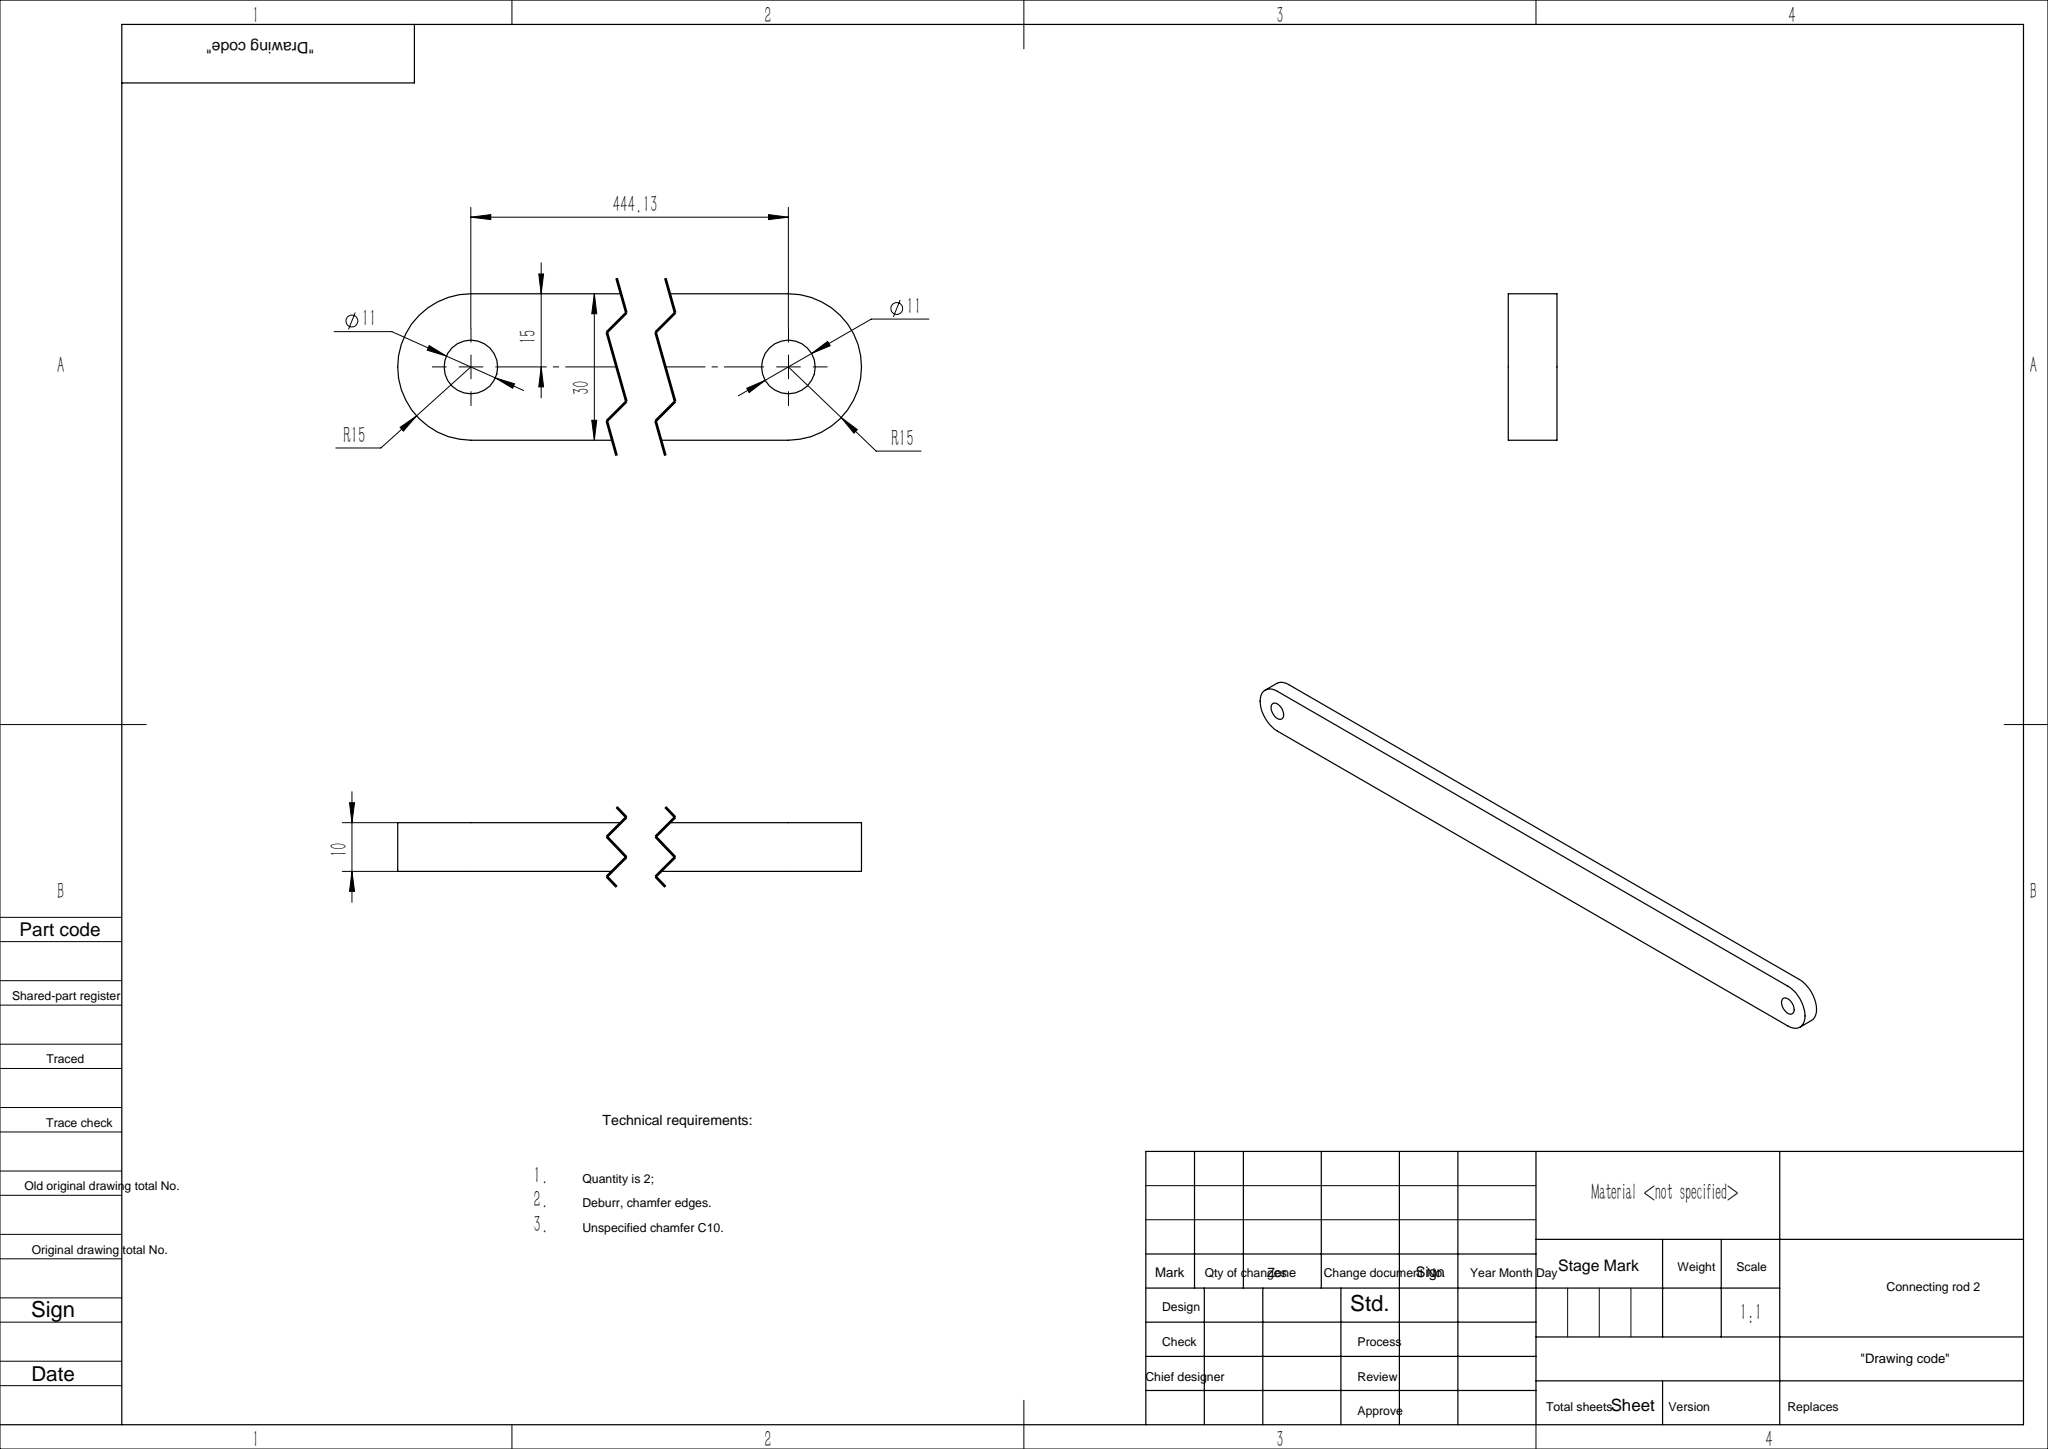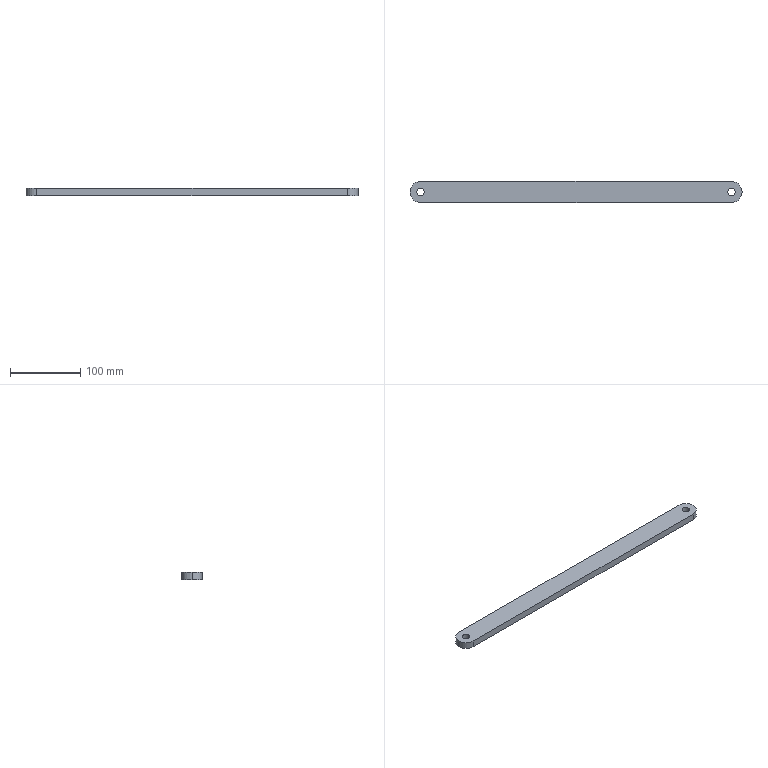Part | SolidWorks | features Extrusion 1, Fillet 1 | 1 solid | 12 faces | box 474.13 x 30 x 10 mm | volume 138407 mm3 | cylinder 8 | plane 4 | commonest cylinder face diameters 11 x4 30 x4
STEP:
#1=CARTESIAN_POINT('',(438.63,0.,10.));
#2=VERTEX_POINT('',#1);
#3=CARTESIAN_POINT('',(449.63,0.,10.));
#4=VERTEX_POINT('',#3);
#5=CARTESIAN_POINT('',(444.13,0.,10.));
#6=DIRECTION('',(0.,0.,1.));
#7=DIRECTION('',(1.,0.,0.));
#8=AXIS2_PLACEMENT_3D('',#5,#6,#7);
#9=CIRCLE('',#8,5.5);
#10=EDGE_CURVE('',#2,#4,#9,.T.);
#11=ORIENTED_EDGE('',*,*,#10,.T.);
#12=CARTESIAN_POINT('',(449.63,0.,0.));
#13=VERTEX_POINT('',#12);
#14=CARTESIAN_POINT('',(449.63,0.,10.));
#15=DIRECTION('',(0.,0.,-1.));
#16=VECTOR('',#15,1000.);
#17=LINE('',#14,#16);
#18=EDGE_CURVE('',#4,#13,#17,.T.);
#19=ORIENTED_EDGE('',*,*,#18,.T.);
#20=CARTESIAN_POINT('',(438.63,0.,0.));
#21=VERTEX_POINT('',#20);
#22=CARTESIAN_POINT('',(444.13,0.,0.));
#23=DIRECTION('',(0.,0.,1.));
#24=DIRECTION('',(1.,0.,0.));
#25=AXIS2_PLACEMENT_3D('',#22,#23,#24);
#26=CIRCLE('',#25,5.5);
#27=EDGE_CURVE('',#21,#13,#26,.T.);
#28=ORIENTED_EDGE('',*,*,#27,.F.);
#29=CARTESIAN_POINT('',(438.63,0.,10.));
#30=DIRECTION('',(0.,0.,-1.));
#31=VECTOR('',#30,1000.);
#32=LINE('',#29,#31);
#33=EDGE_CURVE('',#2,#21,#32,.T.);
#34=ORIENTED_EDGE('',*,*,#33,.F.);
#35=EDGE_LOOP('',(#11,#19,#28,#34));
#36=FACE_OUTER_BOUND('',#35,.T.);
#37=CARTESIAN_POINT('',(444.13,0.,10.));
#38=DIRECTION('',(0.,0.,-1.));
#39=DIRECTION('',(-1.,0.,0.));
#40=AXIS2_PLACEMENT_3D('',#37,#38,#39);
#41=CYLINDRICAL_SURFACE('',#40,5.5);
#42=ADVANCED_FACE('',(#36),#41,.F.);
#43=CARTESIAN_POINT('',(-5.5,0.,10.));
#44=VERTEX_POINT('',#43);
#45=CARTESIAN_POINT('',(5.5,0.,10.));
#46=VERTEX_POINT('',#45);
#47=CARTESIAN_POINT('',(0.,0.,10.));
#48=DIRECTION('',(0.,0.,1.));
#49=DIRECTION('',(1.,0.,0.));
#50=AXIS2_PLACEMENT_3D('',#47,#48,#49);
#51=CIRCLE('',#50,5.5);
#52=EDGE_CURVE('',#44,#46,#51,.T.);
#53=ORIENTED_EDGE('',*,*,#52,.T.);
#54=CARTESIAN_POINT('',(5.5,0.,0.));
#55=VERTEX_POINT('',#54);
#56=CARTESIAN_POINT('',(5.5,0.,10.));
#57=DIRECTION('',(0.,0.,-1.));
#58=VECTOR('',#57,1000.);
#59=LINE('',#56,#58);
#60=EDGE_CURVE('',#46,#55,#59,.T.);
#61=ORIENTED_EDGE('',*,*,#60,.T.);
#62=CARTESIAN_POINT('',(-5.5,0.,0.));
#63=VERTEX_POINT('',#62);
#64=CARTESIAN_POINT('',(0.,0.,0.));
#65=DIRECTION('',(0.,0.,1.));
#66=DIRECTION('',(1.,0.,0.));
#67=AXIS2_PLACEMENT_3D('',#64,#65,#66);
#68=CIRCLE('',#67,5.5);
#69=EDGE_CURVE('',#63,#55,#68,.T.);
#70=ORIENTED_EDGE('',*,*,#69,.F.);
#71=CARTESIAN_POINT('',(-5.5,0.,10.));
#72=DIRECTION('',(0.,0.,-1.));
#73=VECTOR('',#72,1000.);
#74=LINE('',#71,#73);
#75=EDGE_CURVE('',#44,#63,#74,.T.);
#76=ORIENTED_EDGE('',*,*,#75,.F.);
#77=EDGE_LOOP('',(#53,#61,#70,#76));
#78=FACE_OUTER_BOUND('',#77,.T.);
#79=CARTESIAN_POINT('',(0.,0.,10.));
#80=DIRECTION('',(0.,0.,-1.));
#81=DIRECTION('',(-1.,0.,0.));
#82=AXIS2_PLACEMENT_3D('',#79,#80,#81);
#83=CYLINDRICAL_SURFACE('',#82,5.5);
#84=ADVANCED_FACE('',(#78),#83,.F.);
#85=ORIENTED_EDGE('',*,*,#52,.F.);
#86=CARTESIAN_POINT('',(0.,0.,10.));
#87=DIRECTION('',(0.,0.,1.));
#88=DIRECTION('',(1.,0.,0.));
#89=AXIS2_PLACEMENT_3D('',#86,#87,#88);
#90=CIRCLE('',#89,5.5);
#91=EDGE_CURVE('',#46,#44,#90,.T.);
#92=ORIENTED_EDGE('',*,*,#91,.F.);
#93=EDGE_LOOP('',(#85,#92));
#94=FACE_BOUND('',#93,.T.);
#95=CARTESIAN_POINT('',(0.,15.,10.));
#96=VERTEX_POINT('',#95);
#97=CARTESIAN_POINT('',(-15.,0.,10.));
#98=VERTEX_POINT('',#97);
#99=CARTESIAN_POINT('',(0.,0.,10.));
#100=DIRECTION('',(0.,0.,1.));
#101=DIRECTION('',(1.,0.,0.));
#102=AXIS2_PLACEMENT_3D('',#99,#100,#101);
#103=CIRCLE('',#102,15.);
#104=EDGE_CURVE('',#96,#98,#103,.T.);
#105=ORIENTED_EDGE('',*,*,#104,.T.);
#106=CARTESIAN_POINT('',(0.,-15.,10.));
#107=VERTEX_POINT('',#106);
#108=CARTESIAN_POINT('',(0.,0.,10.));
#109=DIRECTION('',(0.,0.,1.));
#110=DIRECTION('',(1.,0.,0.));
#111=AXIS2_PLACEMENT_3D('',#108,#109,#110);
#112=CIRCLE('',#111,15.);
#113=EDGE_CURVE('',#98,#107,#112,.T.);
#114=ORIENTED_EDGE('',*,*,#113,.T.);
#115=CARTESIAN_POINT('',(444.13,-15.,10.));
#116=VERTEX_POINT('',#115);
#117=CARTESIAN_POINT('',(0.,-15.,10.));
#118=DIRECTION('',(1.,0.,0.));
#119=VECTOR('',#118,1000.);
#120=LINE('',#117,#119);
#121=EDGE_CURVE('',#107,#116,#120,.T.);
#122=ORIENTED_EDGE('',*,*,#121,.T.);
#123=CARTESIAN_POINT('',(459.13,0.,10.));
#124=VERTEX_POINT('',#123);
#125=CARTESIAN_POINT('',(444.13,0.,10.));
#126=DIRECTION('',(0.,0.,1.));
#127=DIRECTION('',(1.,0.,0.));
#128=AXIS2_PLACEMENT_3D('',#125,#126,#127);
#129=CIRCLE('',#128,15.);
#130=EDGE_CURVE('',#116,#124,#129,.T.);
#131=ORIENTED_EDGE('',*,*,#130,.T.);
#132=CARTESIAN_POINT('',(444.13,15.,10.));
#133=VERTEX_POINT('',#132);
#134=CARTESIAN_POINT('',(444.13,0.,10.));
#135=DIRECTION('',(0.,0.,1.));
#136=DIRECTION('',(1.,0.,0.));
#137=AXIS2_PLACEMENT_3D('',#134,#135,#136);
#138=CIRCLE('',#137,15.);
#139=EDGE_CURVE('',#124,#133,#138,.T.);
#140=ORIENTED_EDGE('',*,*,#139,.T.);
#141=CARTESIAN_POINT('',(444.13,15.,10.));
#142=DIRECTION('',(-1.,0.,0.));
#143=VECTOR('',#142,1000.);
#144=LINE('',#141,#143);
#145=EDGE_CURVE('',#133,#96,#144,.T.);
#146=ORIENTED_EDGE('',*,*,#145,.T.);
#147=EDGE_LOOP('',(#105,#114,#122,#131,#140,#146));
#148=FACE_OUTER_BOUND('',#147,.T.);
#149=ORIENTED_EDGE('',*,*,#10,.F.);
#150=CARTESIAN_POINT('',(444.13,0.,10.));
#151=DIRECTION('',(0.,0.,1.));
#152=DIRECTION('',(1.,0.,0.));
#153=AXIS2_PLACEMENT_3D('',#150,#151,#152);
#154=CIRCLE('',#153,5.5);
#155=EDGE_CURVE('',#4,#2,#154,.T.);
#156=ORIENTED_EDGE('',*,*,#155,.F.);
#157=EDGE_LOOP('',(#149,#156));
#158=FACE_BOUND('',#157,.T.);
#159=CARTESIAN_POINT('',(0.,0.,10.));
#160=DIRECTION('',(0.,0.,1.));
#161=DIRECTION('',(1.,0.,0.));
#162=AXIS2_PLACEMENT_3D('',#159,#160,#161);
#163=PLANE('',#162);
#164=ADVANCED_FACE('',(#94,#148,#158),#163,.T.);
#165=ORIENTED_EDGE('',*,*,#69,.T.);
#166=CARTESIAN_POINT('',(0.,0.,0.));
#167=DIRECTION('',(0.,0.,1.));
#168=DIRECTION('',(1.,0.,0.));
#169=AXIS2_PLACEMENT_3D('',#166,#167,#168);
#170=CIRCLE('',#169,5.5);
#171=EDGE_CURVE('',#55,#63,#170,.T.);
#172=ORIENTED_EDGE('',*,*,#171,.T.);
#173=EDGE_LOOP('',(#165,#172));
#174=FACE_BOUND('',#173,.T.);
#175=CARTESIAN_POINT('',(0.,-15.,0.));
#176=VERTEX_POINT('',#175);
#177=CARTESIAN_POINT('',(444.13,-15.,0.));
#178=VERTEX_POINT('',#177);
#179=CARTESIAN_POINT('',(0.,-15.,0.));
#180=DIRECTION('',(1.,0.,0.));
#181=VECTOR('',#180,1000.);
#182=LINE('',#179,#181);
#183=EDGE_CURVE('',#176,#178,#182,.T.);
#184=ORIENTED_EDGE('',*,*,#183,.F.);
#185=CARTESIAN_POINT('',(-15.,0.,0.));
#186=VERTEX_POINT('',#185);
#187=CARTESIAN_POINT('',(0.,0.,0.));
#188=DIRECTION('',(0.,0.,-1.));
#189=DIRECTION('',(1.,0.,0.));
#190=AXIS2_PLACEMENT_3D('',#187,#188,#189);
#191=CIRCLE('',#190,15.);
#192=EDGE_CURVE('',#176,#186,#191,.T.);
#193=ORIENTED_EDGE('',*,*,#192,.T.);
#194=CARTESIAN_POINT('',(0.,15.,0.));
#195=VERTEX_POINT('',#194);
#196=CARTESIAN_POINT('',(0.,0.,0.));
#197=DIRECTION('',(0.,0.,-1.));
#198=DIRECTION('',(1.,0.,0.));
#199=AXIS2_PLACEMENT_3D('',#196,#197,#198);
#200=CIRCLE('',#199,15.);
#201=EDGE_CURVE('',#186,#195,#200,.T.);
#202=ORIENTED_EDGE('',*,*,#201,.T.);
#203=CARTESIAN_POINT('',(444.13,15.,0.));
#204=VERTEX_POINT('',#203);
#205=CARTESIAN_POINT('',(0.,15.,0.));
#206=DIRECTION('',(-1.,0.,0.));
#207=VECTOR('',#206,1000.);
#208=LINE('',#205,#207);
#209=EDGE_CURVE('',#204,#195,#208,.T.);
#210=ORIENTED_EDGE('',*,*,#209,.F.);
#211=CARTESIAN_POINT('',(459.13,0.,0.));
#212=VERTEX_POINT('',#211);
#213=CARTESIAN_POINT('',(444.13,0.,0.));
#214=DIRECTION('',(0.,0.,-1.));
#215=DIRECTION('',(1.,0.,0.));
#216=AXIS2_PLACEMENT_3D('',#213,#214,#215);
#217=CIRCLE('',#216,15.);
#218=EDGE_CURVE('',#204,#212,#217,.T.);
#219=ORIENTED_EDGE('',*,*,#218,.T.);
#220=CARTESIAN_POINT('',(444.13,0.,0.));
#221=DIRECTION('',(0.,0.,-1.));
#222=DIRECTION('',(1.,0.,0.));
#223=AXIS2_PLACEMENT_3D('',#220,#221,#222);
#224=CIRCLE('',#223,15.);
#225=EDGE_CURVE('',#212,#178,#224,.T.);
#226=ORIENTED_EDGE('',*,*,#225,.T.);
#227=EDGE_LOOP('',(#184,#193,#202,#210,#219,#226));
#228=FACE_OUTER_BOUND('',#227,.T.);
#229=ORIENTED_EDGE('',*,*,#27,.T.);
#230=CARTESIAN_POINT('',(444.13,0.,0.));
#231=DIRECTION('',(0.,0.,1.));
#232=DIRECTION('',(1.,0.,0.));
#233=AXIS2_PLACEMENT_3D('',#230,#231,#232);
#234=CIRCLE('',#233,5.5);
#235=EDGE_CURVE('',#13,#21,#234,.T.);
#236=ORIENTED_EDGE('',*,*,#235,.T.);
#237=EDGE_LOOP('',(#229,#236));
#238=FACE_BOUND('',#237,.T.);
#239=CARTESIAN_POINT('',(0.,0.,0.));
#240=DIRECTION('',(0.,0.,1.));
#241=DIRECTION('',(1.,0.,0.));
#242=AXIS2_PLACEMENT_3D('',#239,#240,#241);
#243=PLANE('',#242);
#244=ADVANCED_FACE('',(#174,#228,#238),#243,.F.);
#245=ORIENTED_EDGE('',*,*,#209,.T.);
#246=CARTESIAN_POINT('',(0.,15.,10.));
#247=DIRECTION('',(0.,0.,1.));
#248=VECTOR('',#247,1000.);
#249=LINE('',#246,#248);
#250=EDGE_CURVE('',#195,#96,#249,.T.);
#251=ORIENTED_EDGE('',*,*,#250,.T.);
#252=ORIENTED_EDGE('',*,*,#145,.F.);
#253=CARTESIAN_POINT('',(444.13,15.,10.));
#254=DIRECTION('',(0.,0.,-1.));
#255=VECTOR('',#254,1000.);
#256=LINE('',#253,#255);
#257=EDGE_CURVE('',#133,#204,#256,.T.);
#258=ORIENTED_EDGE('',*,*,#257,.T.);
#259=EDGE_LOOP('',(#245,#251,#252,#258));
#260=FACE_OUTER_BOUND('',#259,.T.);
#261=CARTESIAN_POINT('',(0.,15.,10.));
#262=DIRECTION('',(0.,-1.,0.));
#263=DIRECTION('',(0.,0.,-1.));
#264=AXIS2_PLACEMENT_3D('',#261,#262,#263);
#265=PLANE('',#264);
#266=ADVANCED_FACE('',(#260),#265,.F.);
#267=ORIENTED_EDGE('',*,*,#121,.F.);
#268=CARTESIAN_POINT('',(0.,-15.,10.));
#269=DIRECTION('',(0.,0.,-1.));
#270=VECTOR('',#269,1000.);
#271=LINE('',#268,#270);
#272=EDGE_CURVE('',#107,#176,#271,.T.);
#273=ORIENTED_EDGE('',*,*,#272,.T.);
#274=ORIENTED_EDGE('',*,*,#183,.T.);
#275=CARTESIAN_POINT('',(444.13,-15.,10.));
#276=DIRECTION('',(0.,0.,1.));
#277=VECTOR('',#276,1000.);
#278=LINE('',#275,#277);
#279=EDGE_CURVE('',#178,#116,#278,.T.);
#280=ORIENTED_EDGE('',*,*,#279,.T.);
#281=EDGE_LOOP('',(#267,#273,#274,#280));
#282=FACE_OUTER_BOUND('',#281,.T.);
#283=CARTESIAN_POINT('',(0.,-15.,10.));
#284=DIRECTION('',(0.,1.,0.));
#285=DIRECTION('',(0.,0.,1.));
#286=AXIS2_PLACEMENT_3D('',#283,#284,#285);
#287=PLANE('',#286);
#288=ADVANCED_FACE('',(#282),#287,.F.);
#289=ORIENTED_EDGE('',*,*,#60,.F.);
#290=ORIENTED_EDGE('',*,*,#91,.T.);
#291=ORIENTED_EDGE('',*,*,#75,.T.);
#292=ORIENTED_EDGE('',*,*,#171,.F.);
#293=EDGE_LOOP('',(#289,#290,#291,#292));
#294=FACE_OUTER_BOUND('',#293,.T.);
#295=CARTESIAN_POINT('',(0.,0.,10.));
#296=DIRECTION('',(0.,0.,-1.));
#297=DIRECTION('',(-1.,0.,0.));
#298=AXIS2_PLACEMENT_3D('',#295,#296,#297);
#299=CYLINDRICAL_SURFACE('',#298,5.5);
#300=ADVANCED_FACE('',(#294),#299,.F.);
#301=ORIENTED_EDGE('',*,*,#18,.F.);
#302=ORIENTED_EDGE('',*,*,#155,.T.);
#303=ORIENTED_EDGE('',*,*,#33,.T.);
#304=ORIENTED_EDGE('',*,*,#235,.F.);
#305=EDGE_LOOP('',(#301,#302,#303,#304));
#306=FACE_OUTER_BOUND('',#305,.T.);
#307=CARTESIAN_POINT('',(444.13,0.,10.));
#308=DIRECTION('',(0.,0.,-1.));
#309=DIRECTION('',(-1.,0.,0.));
#310=AXIS2_PLACEMENT_3D('',#307,#308,#309);
#311=CYLINDRICAL_SURFACE('',#310,5.5);
#312=ADVANCED_FACE('',(#306),#311,.F.);
#313=CARTESIAN_POINT('',(-15.,0.,10.));
#314=DIRECTION('',(0.,0.,-1.));
#315=VECTOR('',#314,1000.);
#316=LINE('',#313,#315);
#317=EDGE_CURVE('',#98,#186,#316,.T.);
#318=ORIENTED_EDGE('',*,*,#317,.F.);
#319=ORIENTED_EDGE('',*,*,#104,.F.);
#320=ORIENTED_EDGE('',*,*,#250,.F.);
#321=ORIENTED_EDGE('',*,*,#201,.F.);
#322=EDGE_LOOP('',(#318,#319,#320,#321));
#323=FACE_OUTER_BOUND('',#322,.T.);
#324=CARTESIAN_POINT('',(0.,0.,10.));
#325=DIRECTION('',(0.,0.,-1.));
#326=DIRECTION('',(-1.,0.,0.));
#327=AXIS2_PLACEMENT_3D('',#324,#325,#326);
#328=CYLINDRICAL_SURFACE('',#327,15.);
#329=ADVANCED_FACE('',(#323),#328,.T.);
#330=ORIENTED_EDGE('',*,*,#113,.F.);
#331=ORIENTED_EDGE('',*,*,#317,.T.);
#332=ORIENTED_EDGE('',*,*,#192,.F.);
#333=ORIENTED_EDGE('',*,*,#272,.F.);
#334=EDGE_LOOP('',(#330,#331,#332,#333));
#335=FACE_OUTER_BOUND('',#334,.T.);
#336=CARTESIAN_POINT('',(0.,0.,10.));
#337=DIRECTION('',(0.,0.,-1.));
#338=DIRECTION('',(-1.,0.,0.));
#339=AXIS2_PLACEMENT_3D('',#336,#337,#338);
#340=CYLINDRICAL_SURFACE('',#339,15.);
#341=ADVANCED_FACE('',(#335),#340,.T.);
#342=ORIENTED_EDGE('',*,*,#257,.F.);
#343=ORIENTED_EDGE('',*,*,#139,.F.);
#344=CARTESIAN_POINT('',(459.13,0.,10.));
#345=DIRECTION('',(0.,0.,1.));
#346=VECTOR('',#345,1000.);
#347=LINE('',#344,#346);
#348=EDGE_CURVE('',#212,#124,#347,.T.);
#349=ORIENTED_EDGE('',*,*,#348,.F.);
#350=ORIENTED_EDGE('',*,*,#218,.F.);
#351=EDGE_LOOP('',(#342,#343,#349,#350));
#352=FACE_OUTER_BOUND('',#351,.T.);
#353=CARTESIAN_POINT('',(444.13,0.,10.));
#354=DIRECTION('',(0.,0.,-1.));
#355=DIRECTION('',(-1.,0.,0.));
#356=AXIS2_PLACEMENT_3D('',#353,#354,#355);
#357=CYLINDRICAL_SURFACE('',#356,15.);
#358=ADVANCED_FACE('',(#352),#357,.T.);
#359=ORIENTED_EDGE('',*,*,#130,.F.);
#360=ORIENTED_EDGE('',*,*,#279,.F.);
#361=ORIENTED_EDGE('',*,*,#225,.F.);
#362=ORIENTED_EDGE('',*,*,#348,.T.);
#363=EDGE_LOOP('',(#359,#360,#361,#362));
#364=FACE_OUTER_BOUND('',#363,.T.);
#365=CARTESIAN_POINT('',(444.13,0.,10.));
#366=DIRECTION('',(0.,0.,-1.));
#367=DIRECTION('',(-1.,0.,0.));
#368=AXIS2_PLACEMENT_3D('',#365,#366,#367);
#369=CYLINDRICAL_SURFACE('',#368,15.);
#370=ADVANCED_FACE('',(#364),#369,.T.);
#371=CLOSED_SHELL('',(#42,#84,#164,#244,#266,#288,#300,#312,#329,#341,#358,#370));
#372=MANIFOLD_SOLID_BREP('',#371);
#373=CARTESIAN_POINT('',(0.,0.,0.));
#374=DIRECTION('',(0.,0.,1.));
#375=DIRECTION('',(1.,0.,0.));
#376=AXIS2_PLACEMENT_3D('',#373,#374,#375);
#377=(LENGTH_UNIT()NAMED_UNIT(*)SI_UNIT(.MILLI.,.METRE.));
#378=UNCERTAINTY_MEASURE_WITH_UNIT(LENGTH_MEASURE(0.00001),#377,'','');
#379=(NAMED_UNIT(*)PLANE_ANGLE_UNIT()SI_UNIT($,.RADIAN.));
#380=(NAMED_UNIT(*)SI_UNIT($,.STERADIAN.)SOLID_ANGLE_UNIT());
#381=(GEOMETRIC_REPRESENTATION_CONTEXT(3)GLOBAL_UNCERTAINTY_ASSIGNED_CONTEXT((#378))GLOBAL_UNIT_ASSIGNED_CONTEXT((#377,#379,#380))REPRESENTATION_CONTEXT('',''));
#382=ADVANCED_BREP_SHAPE_REPRESENTATION('',(#372,#376),#381);